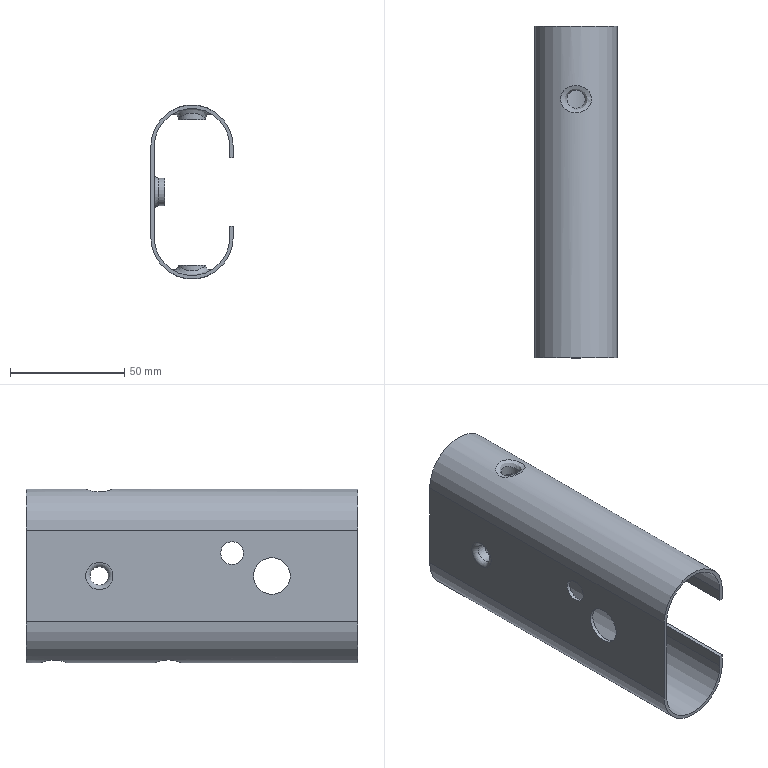Part | STEP file | 6100105L | 1 solid | 36 faces | box 36 x 145 x 76 mm | volume 34893 mm3 | cylinder 14 | plane 14 | spline 6 | torus 2 | commonest cylinder face diameters 8 x4 12 x4 33 x2 36 x2 10 x1 16 x1